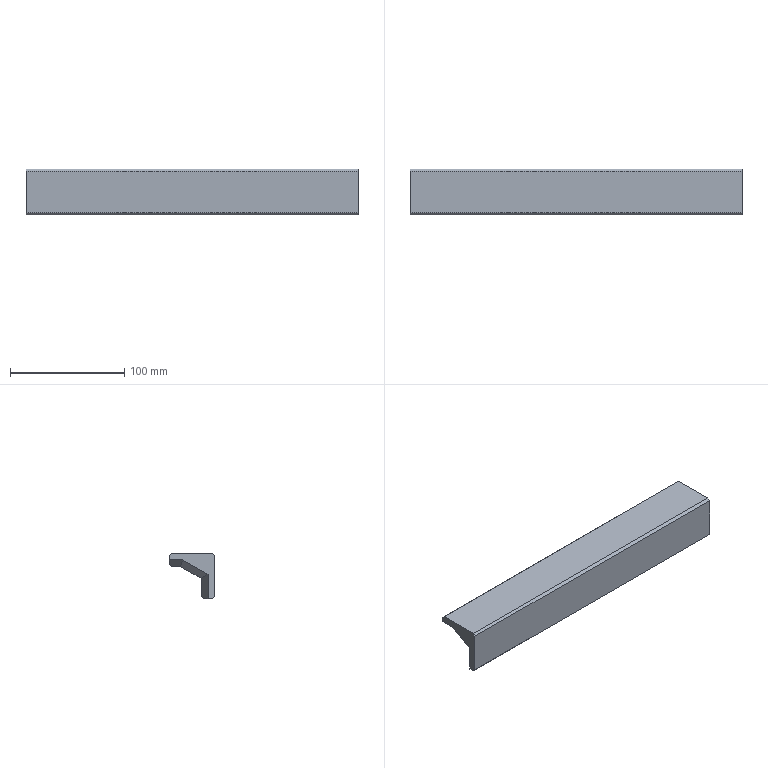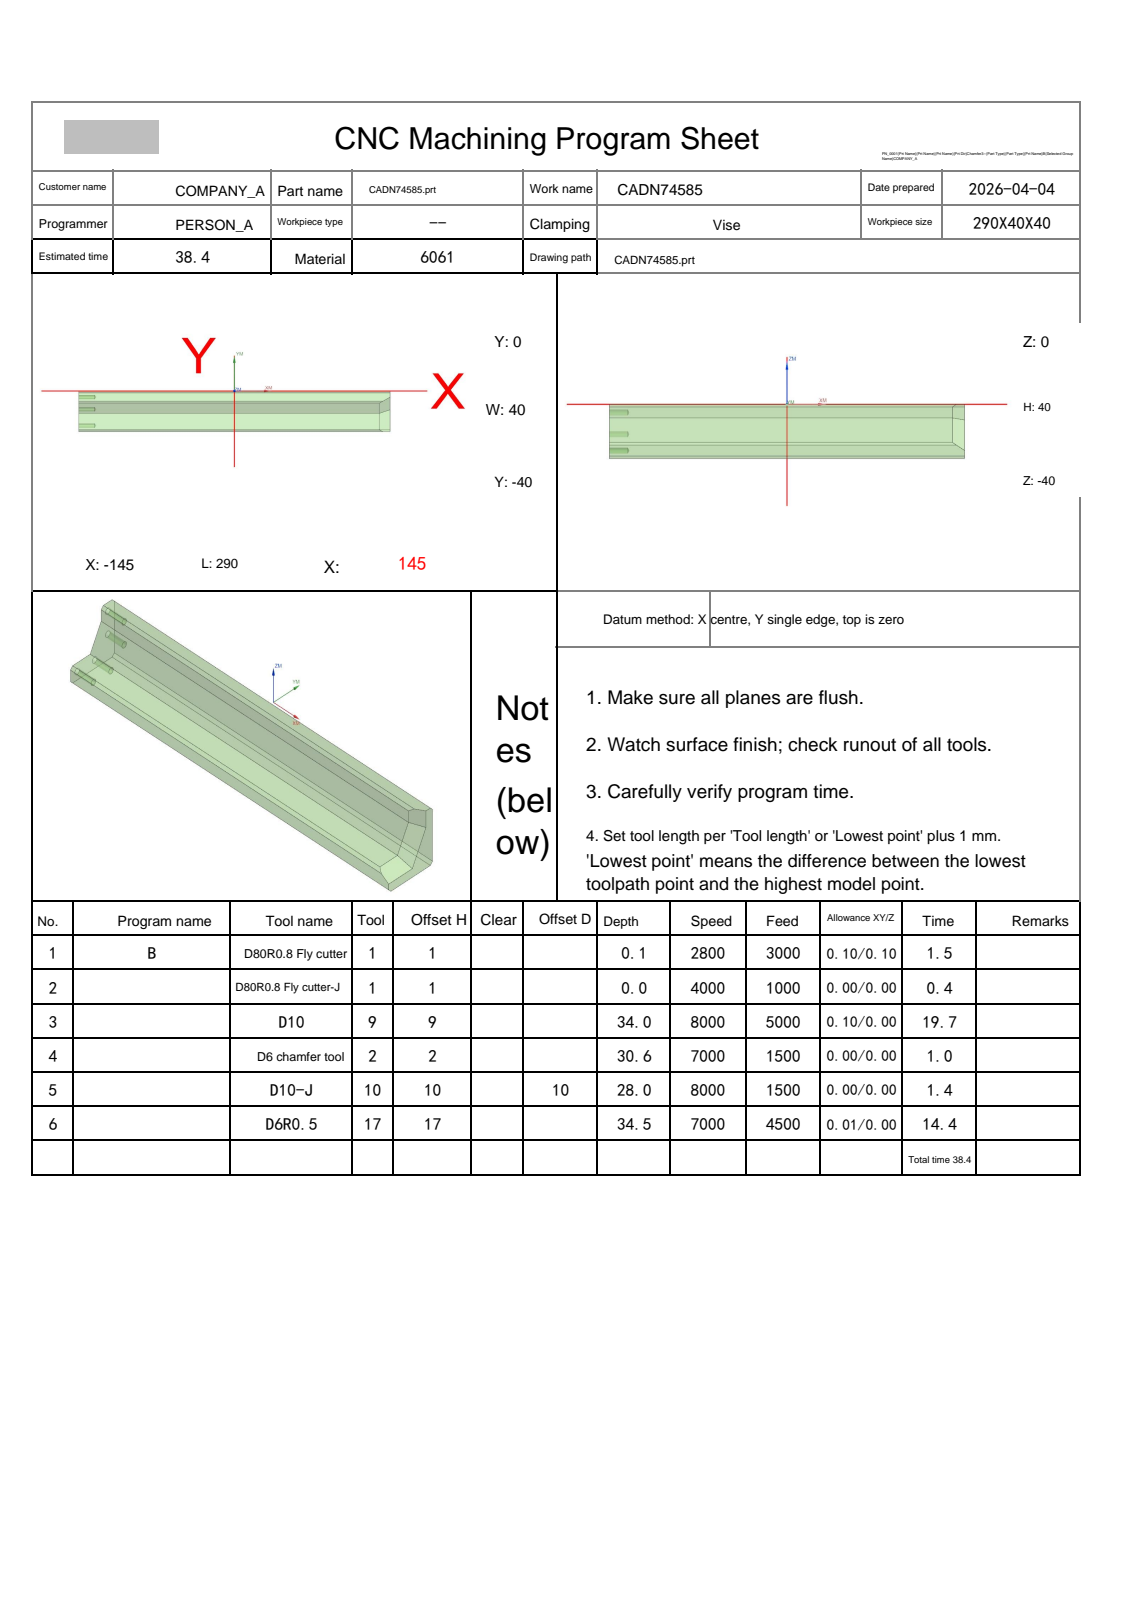NC program | NX | posted by the shop | part box 290 x 40 x 40 mm
Lines 110 to 1353 of 6846:
N3 T09 M06
(D10  D=10. R=0. H=09 ce=0.10 di=0.10)
G00 G90 G54 X8.423 Y-52.151 M03 S8000
G43 H09 Z14.5
M08
Z.702
G01 Z-.498 F5000.
Y-50.
G03 X1.423 Y-43. I-7. J0.0
G01 X-145.08
Y-42.864
Y-27.494
Y-27.051
Y-17.648
Y-17.039
Y-16.914
Y-15.639
X-138.08 Y-15.64
X137.385
G03 X140.127 Y-14.871 I-.14 J5.778
G01 X141. Y-14.348
X141.14 Y-14.264
X141.913 Y-13.8
X147.633 Y-10.368
G03 X147.945 Y-10.165 I-2.603 J4.338
G01 X147.961 Y-10.212
Y-11.804
Y-21.827
X147.994 Y-21.852
X148. Y-21.848
Y-40.08
X143.456
X143.382 Y-40.73
G02 X142.478 Y-43. I-5.022 J.686
G01 X-.563
G02 X-1.375 Y-42.582 I.001 J1.
G01 X-5.778 Y-36.418
G03 X-6.591 Y-36. I-.813 J-.582
G01 X-137.083
G02 X-138.08 Y-35.004 I.004 J1.
G01 Y-27.495
Y-27.052
Y-23.636
G02 X-137.084 Y-22.64 I1. J-.004
G01 X137.47
G03 X139.803 Y-22.383 I-.227 J12.778
G01 X140. Y-22.363
G02 X141. Y-23.359 I0.0 J-1.
G01 Y-32.868
G02 X140.435 Y-33.765 I-1. J.004
G03 X138.046 Y-35.638 I3.021 J-6.314
G02 X137.279 Y-36. I-.77 J.638
G01 X-.914
G02 X-1.619 Y-35.708 I.001 J1.
G01 X-5.534 Y-31.793
G03 X-6.241 Y-31.5 I-.707 J-.707
G01 X-132.584
G02 X-133.58 Y-30.504 I.004 J1.
G01 Y-28.135
G02 X-132.584 Y-27.14 I1. J-.004
G01 X135.504
G02 X136.5 Y-28.135 I-.004 J-1.
G01 Y-30.443
G02 X136.14 Y-31.207 I-1. J.004
G01 X136.065 Y-31.269
G02 X135.43 Y-31.5 I-.639 J.769
G01 X-3.577
X-4.077
G03 X-11.077 Y-38.5 I0.0 J-7.
G01 Y-52.151
Z.702
G00 Z3.
G01 X8.423 F6000.
G00 Z.204
G01 Z-.996 F5000.
Y-50.
G03 X1.423 Y-43. I-7. J0.0
G01 X-145.08
Y-42.864
Y-27.494
Y-27.051
Y-17.648
Y-16.914
Y-16.136
X-138.08 Y-16.138
X136.399
X136.45
G03 X139.297 Y-15.37 I0.0 J5.655
G01 X141. Y-14.348
X147.633 Y-10.368
G03 X147.945 Y-10.165 I-2.603 J4.338
G01 X147.961 Y-10.212
Y-11.804
Y-21.827
X147.994 Y-21.852
X148. Y-21.848
Y-40.08
X143.456
X143.382 Y-40.73
G02 X142.478 Y-43. I-5.022 J.686
G01 X-3.577
G02 X-4.548 Y-42.238 I0.0 J1.
G01 X-5.89 Y-36.761
G03 X-6.861 Y-36. I-.971 J-.239
G01 X-137.084
G02 X-138.08 Y-35.004 I.004 J1.
G01 Y-27.495
Y-27.052
Y-24.134
G02 X-137.084 Y-23.138 I1. J-.004
G01 X136.34
X136.45
G03 X139.744 Y-22.702 I0.0 J12.655
G02 X140. Y-22.669 I.256 J-.967
X141. Y-23.665 I0.0 J-1.
G01 Y-32.869
G02 X140.435 Y-33.765 I-1. J.004
G03 X138.046 Y-35.638 I3.021 J-6.315
G02 X137.28 Y-36. I-.77 J.638
G01 X-.914
G02 X-1.619 Y-35.708 I.001 J1.
G01 X-5.534 Y-31.793
G03 X-6.241 Y-31.5 I-.707 J-.707
G01 X-132.585
G02 X-133.58 Y-30.505 I.005 J1.
G01 Y-28.633
G02 X-132.585 Y-27.638 I1. J-.005
G01 X135.505
G02 X136.5 Y-28.633 I-.005 J-1.
G01 Y-30.443
G02 X136.14 Y-31.207 I-1. J.005
G01 X136.065 Y-31.269
G02 X135.431 Y-31.5 I-.639 J.769
G01 X-3.577
X-4.077
G03 X-11.077 Y-38.5 I0.0 J-7.
G01 Y-52.151
Z.204
G00 Z2.502
G01 X8.423 F6000.
G00 Z-.295
G01 Z-1.495 F5000.
Y-50.
G03 X1.423 Y-43. I-7. J0.0
G01 X-145.08
Y-42.864
Y-27.494
Y-27.051
Y-18.035
Y-17.648
Y-16.914
Y-16.634
X-138.08 Y-16.636
X135.724
G03 X138.466 Y-15.868 I-.016 J5.333
G01 X141. Y-14.348
X147.633 Y-10.368
G03 X147.945 Y-10.165 I-2.603 J4.338
G01 X147.948 Y-10.168
X147.961 Y-10.212
Y-11.804
Y-21.827
X147.994 Y-21.852
X148. Y-21.848
Y-40.08
X143.456
X143.382 Y-40.73
G02 X142.478 Y-43. I-5.022 J.686
G01 X-3.577
G02 X-4.548 Y-42.238 I0.0 J1.
G01 X-5.89 Y-36.761
G03 X-6.861 Y-36. I-.971 J-.239
G01 X-137.084
G02 X-138.08 Y-35.004 I.004 J1.
G01 Y-27.495
Y-27.052
Y-24.632
G02 X-137.084 Y-23.636 I1. J-.004
G01 X135.735
G03 X139.682 Y-22.978 I-.026 J12.333
G02 X140. Y-22.927 I.318 J-.948
X141. Y-23.922 I0.0 J-1.
G01 Y-32.869
G02 X140.436 Y-33.765 I-1. J.004
G03 X138.046 Y-35.638 I3.021 J-6.315
G02 X137.28 Y-36. I-.77 J.638
G01 X-.914
G02 X-1.619 Y-35.708 I.001 J1.
G01 X-5.534 Y-31.793
G03 X-6.241 Y-31.5 I-.707 J-.707
G01 X-132.585
G02 X-133.58 Y-30.505 I.005 J1.
G01 Y-29.131
G02 X-132.585 Y-28.136 I1. J-.005
G01 X135.505
G02 X136.5 Y-29.131 I-.005 J-1.
G01 Y-30.443
G02 X136.14 Y-31.207 I-1. J.005
G01 X136.065 Y-31.269
G02 X135.431 Y-31.5 I-.639 J.769
G01 X-3.577
X-4.077
G03 X-11.077 Y-38.5 I0.0 J-7.
G01 Y-52.151
Z-.295
G00 Z2.004
G01 X8.423 F6000.
G00 Z-.793
G01 Z-1.993 F5000.
Y-50.
G03 X1.423 Y-43. I-7. J0.0
G01 X-145.08
Y-42.864
Y-27.494
Y-27.051
Y-17.648
Y-17.449
Y-17.099
X-138.08 Y-17.1
X134.978
X134.983
G03 X137.636 Y-16.366 I0.0 J5.164
G01 X138.466 Y-15.868
X141. Y-14.348
X147.633 Y-10.368
G03 X147.945 Y-10.165 I-2.603 J4.338
G01 X147.961 Y-10.212
Y-11.804
Y-21.827
X147.994 Y-21.852
X148. Y-21.848
Y-40.08
X143.456
X143.382 Y-40.73
G02 X142.478 Y-43. I-5.022 J.686
G01 X-3.577
G02 X-4.548 Y-42.238 I0.0 J1.
G01 X-5.89 Y-36.761
G03 X-6.861 Y-36. I-.971 J-.239
G01 X-137.085
G02 X-138.08 Y-35.005 I.005 J1.
G01 Y-27.495
Y-27.052
Y-25.095
G02 X-137.085 Y-24.1 I1. J-.005
G01 X134.975
X134.983
G03 X139.623 Y-23.18 I0.0 J12.164
G02 X140. Y-23.106 I.377 J-.926
X141. Y-24.101 I0.0 J-1.
G01 Y-32.869
G02 X140.436 Y-33.765 I-1. J.005
G03 X138.046 Y-35.638 I3.02 J-6.315
G02 X137.28 Y-36. I-.77 J.638
G01 X-.914
G02 X-1.619 Y-35.708 I.001 J1.
G01 X-5.534 Y-31.793
G03 X-6.241 Y-31.5 I-.707 J-.707
G01 X-132.585
G02 X-133.58 Y-30.505 I.005 J1.
G01 Y-29.595
G02 X-132.585 Y-28.6 I1. J-.005
G01 X134.974
X134.983
G03 X135.476 Y-28.592 I0.0 J16.664
G01 X135.5
G02 X136.5 Y-29.587 I0.0 J-1.
G01 Y-30.444
G02 X136.14 Y-31.207 I-1. J.005
G01 X136.065 Y-31.27
G02 X135.431 Y-31.5 I-.639 J.77
G01 X-3.577
X-4.077
G03 X-11.077 Y-38.5 I0.0 J-7.
G01 Y-52.151
Z-.793
G00 Z1.505
G01 X8.423 F6000.
G00 Z-1.291
G01 Z-2.491 F5000.
Y-50.
G03 X1.423 Y-43. I-7. J0.0
G01 X-145.08
Y-42.864
Y-27.494
Y-27.051
Y-17.648
Y-17.099
X-138.08 Y-17.1
X135.
G03 X137.624 Y-16.373 I0.0 J5.1
G01 X141. Y-14.348
X147.633 Y-10.368
G03 X147.945 Y-10.165 I-2.603 J4.338
G01 X147.961 Y-10.212
Y-11.804
Y-21.827
X147.994 Y-21.852
X148. Y-21.848
Y-40.08
X143.456
X143.382 Y-40.73
G02 X142.478 Y-43. I-5.022 J.686
G01 X-3.577
G02 X-4.548 Y-42.238 I0.0 J1.
G01 X-5.89 Y-36.761
G03 X-6.861 Y-36. I-.971 J-.239
G01 X-137.085
G02 X-138.08 Y-35.005 I.005 J1.
G01 Y-27.495
Y-25.095
G02 X-137.085 Y-24.1 I1. J-.005
G01 X135.
G03 X139.623 Y-23.182 I0.0 J12.1
G02 X140. Y-23.108 I.377 J-.926
X141. Y-24.103 I0.0 J-1.
G01 Y-32.87
G02 X140.436 Y-33.765 I-1. J.005
G03 X138.045 Y-35.638 I3.02 J-6.315
G02 X137.281 Y-36. I-.77 J.638
G01 X-.914
G02 X-1.619 Y-35.708 I.001 J1.
G01 X-5.534 Y-31.793
G03 X-6.241 Y-31.5 I-.707 J-.707
G01 X-132.585
G02 X-133.58 Y-30.505 I.005 J1.
G01 Y-29.595
G02 X-132.585 Y-28.6 I1. J-.005
G01 X135.
G03 X135.477 Y-28.593 I0.0 J16.6
G01 X135.5
G02 X136.5 Y-29.587 I0.0 J-1.
G01 Y-30.444
G02 X136.141 Y-31.207 I-1. J.005
G01 X136.065 Y-31.27
G02 X135.432 Y-31.5 I-.638 J.77
G01 X-3.577
X-4.077
G03 X-11.077 Y-38.5 I0.0 J-7.
G01 Y-52.151
Z-1.291
G00 Z1.007
G01 X8.423 F6000.
G00 Z-1.789
G01 Z-2.989 F5000.
Y-50.
G03 X1.423 Y-43. I-7. J0.0
G01 X-145.08
Y-42.864
Y-27.494
Y-27.051
Y-24.1
Y-17.647
Y-17.099
X-138.08 Y-17.1
X135.
X135.208 Y-17.096
G03 X137.624 Y-16.373 I-.208 J5.096
G01 X141. Y-14.348
X147.633 Y-10.368
G03 X147.945 Y-10.165 I-2.603 J4.338
G01 X147.961 Y-10.212
Y-11.804
Y-21.827
X147.994 Y-21.852
X148. Y-21.848
Y-40.08
X143.456
X143.382 Y-40.73
G02 X142.478 Y-43. I-5.022 J.686
G01 X-3.577
G02 X-4.548 Y-42.238 I0.0 J1.
G01 X-5.89 Y-36.761
G03 X-6.861 Y-36. I-.971 J-.239
G01 X-137.085
G02 X-138.08 Y-35.005 I.005 J1.
G01 Y-27.495
Y-27.052
Y-25.095
G02 X-137.085 Y-24.1 I1. J-.005
G01 X135.493 Y-24.09
G03 X139.623 Y-23.182 I-.493 J12.09
G02 X140. Y-23.108 I.377 J-.926
X141. Y-24.103 I0.0 J-1.
G01 Y-32.87
G02 X140.436 Y-33.764 I-1. J.005
G03 X138.045 Y-35.639 I3.02 J-6.315
G02 X137.281 Y-36. I-.769 J.639
G01 X-.914
G02 X-1.619 Y-35.708 I.001 J1.
G01 X-5.534 Y-31.793
G03 X-6.241 Y-31.5 I-.707 J-.707
G01 X-132.586
G02 X-133.58 Y-30.506 I.006 J1.
G01 Y-29.594
G02 X-132.586 Y-28.6 I1. J-.006
G01 X135.506 Y-28.59
G02 X136.5 Y-29.584 I-.006 J-1.
G01 Y-30.444
G02 X136.141 Y-31.206 I-1. J.006
G01 X136.064 Y-31.27
G02 X135.432 Y-31.5 I-.638 J.77
G01 X-3.577
X-4.077
G03 X-11.077 Y-38.5 I0.0 J-7.
G01 Y-52.151
Z-1.789
G00 Z.509
G01 X8.423 F6000.
G00 Z-2.288
G01 Z-3.488 F5000.
Y-50.
G03 X1.423 Y-43. I-7. J0.0
G01 X-145.08
Y-42.864
Y-27.494
Y-27.051
Y-17.648
Y-17.099
X-138.08 Y-17.1
X135.
G03 X137.624 Y-16.373 I0.0 J5.1
G01 X141. Y-14.348
X147.633 Y-10.368
G03 X147.945 Y-10.165 I-2.603 J4.338
G01 X147.948 Y-10.168
X147.961 Y-10.212
Y-11.804
Y-21.827
X147.994 Y-21.852
X148. Y-21.848
Y-40.08
X143.456
X143.382 Y-40.73
G02 X142.478 Y-43. I-5.022 J.686
G01 X-3.577
G02 X-4.548 Y-42.238 I0.0 J1.
G01 X-5.89 Y-36.761
G03 X-6.861 Y-36. I-.971 J-.239
G01 X-137.085
G02 X-138.08 Y-35.005 I.005 J1.
G01 Y-27.495
Y-27.052
Y-25.095
G02 X-137.085 Y-24.1 I1. J-.005
G01 X135.
G03 X139.623 Y-23.182 I0.0 J12.1
G02 X140. Y-23.108 I.377 J-.926
X141. Y-24.103 I0.0 J-1.
G01 Y-32.87
G02 X140.437 Y-33.764 I-1. J.005
G03 X138.045 Y-35.639 I3.02 J-6.315
G02 X137.281 Y-36. I-.769 J.639
G01 X-.914
G02 X-1.619 Y-35.708 I.001 J1.
G01 X-5.534 Y-31.793
G03 X-6.241 Y-31.5 I-.707 J-.707
G01 X-132.586
G02 X-133.58 Y-30.506 I.006 J1.
G01 Y-29.594
G02 X-132.586 Y-28.6 I1. J-.006
G01 X135.
G03 X135.477 Y-28.593 I0.0 J16.6
G01 X135.5
G02 X136.5 Y-29.587 I0.0 J-1.
G01 Y-30.445
G02 X136.141 Y-31.206 I-1. J.006
G01 X136.064 Y-31.27
G02 X135.432 Y-31.5 I-.638 J.77
G01 X-3.577
X-4.077
G03 X-11.077 Y-38.5 I0.0 J-7.
G01 Y-52.151
Z-2.288
G00 Z.011
G01 X8.423 F6000.
G00 Z-2.786
G01 Z-3.986 F5000.
Y-50.
G03 X1.423 Y-43. I-7. J0.0
G01 X-145.08
Y-42.864
Y-27.494
Y-27.051
Y-17.648
Y-17.099
X-138.08 Y-17.1
X135.
G03 X137.624 Y-16.373 I0.0 J5.1
G01 X141. Y-14.348
X147.633 Y-10.368
G03 X147.945 Y-10.165 I-2.603 J4.338
G01 X147.948 Y-10.168
X147.961 Y-10.212
Y-11.804
Y-21.827
X147.994 Y-21.852
X148. Y-21.848
Y-40.08
X143.456
X143.382 Y-40.73
G02 X142.478 Y-43. I-5.022 J.686
G01 X-3.577
G02 X-4.548 Y-42.238 I0.0 J1.
G01 X-5.89 Y-36.761
G03 X-6.861 Y-36. I-.971 J-.239
G01 X-137.086
G02 X-138.08 Y-35.006 I.006 J1.
G01 Y-27.495
Y-27.052
Y-25.094
G02 X-137.086 Y-24.1 I1. J-.006
G01 X135.
G03 X139.623 Y-23.182 I0.0 J12.1
G02 X140. Y-23.108 I.377 J-.926
X141. Y-24.103 I0.0 J-1.
G01 Y-32.87
G02 X140.437 Y-33.764 I-1. J.006
G03 X138.045 Y-35.639 I3.019 J-6.315
G02 X137.281 Y-36. I-.769 J.639
G01 X-.914
G02 X-1.619 Y-35.708 I.001 J1.
G01 X-5.534 Y-31.793
G03 X-6.241 Y-31.5 I-.707 J-.707
G01 X-132.586
G02 X-133.58 Y-30.506 I.006 J1.
G01 Y-29.594
G02 X-132.586 Y-28.6 I1. J-.006
G01 X135.
G03 X135.478 Y-28.593 I0.0 J16.6
G01 X135.5
G02 X136.5 Y-29.587 I0.0 J-1.
G01 Y-30.445
G02 X136.141 Y-31.206 I-1. J.006
G01 X136.064 Y-31.27
G02 X135.432 Y-31.5 I-.638 J.77
G01 X-3.577
X-4.077
G03 X-11.077 Y-38.5 I0.0 J-7.
G01 Y-52.151
Z-2.786
G00 Z-.488
G01 X8.423 F6000.
G00 Z-3.284
G01 Z-4.484 F5000.
Y-50.
G03 X1.423 Y-43. I-7. J0.0
G01 X-145.08
Y-42.864
Y-27.494
Y-27.051
Y-17.648
Y-17.099
X-138.08 Y-17.1
X135.
G03 X137.624 Y-16.373 I0.0 J5.1
G01 X141. Y-14.348
X147.633 Y-10.368
G03 X147.945 Y-10.165 I-2.603 J4.338
G01 X147.948 Y-10.168
X147.961 Y-10.212
Y-11.804
Y-21.827
X147.994 Y-21.852
X148. Y-21.848
Y-40.08
X143.456
X143.382 Y-40.73
G02 X142.478 Y-43. I-5.022 J.686
G01 X-3.577
G02 X-4.548 Y-42.238 I0.0 J1.
G01 X-5.89 Y-36.761
G03 X-6.861 Y-36. I-.971 J-.239
G01 X-137.086
G02 X-138.08 Y-35.006 I.006 J1.
G01 Y-27.495
Y-27.052
Y-25.094
G02 X-137.086 Y-24.1 I1. J-.006
G01 X135.
G03 X139.624 Y-23.182 I0.0 J12.1
G02 X140. Y-23.108 I.376 J-.926
X141. Y-24.102 I0.0 J-1.
G01 Y-32.871
G02 X140.437 Y-33.764 I-1. J.006
G03 X138.045 Y-35.639 I3.019 J-6.315
G02 X137.282 Y-36. I-.769 J.639
G01 X-.914
G02 X-1.619 Y-35.708 I.001 J1.
G01 X-5.534 Y-31.793
G03 X-6.241 Y-31.5 I-.707 J-.707
G01 X-132.586
G02 X-133.58 Y-30.506 I.006 J1.
G01 Y-29.594
G02 X-132.586 Y-28.6 I1. J-.006
G01 X135.
G03 X135.478 Y-28.593 I0.0 J16.6
G01 X135.5
G02 X136.5 Y-29.586 I0.0 J-1.
G01 Y-30.445
G02 X136.141 Y-31.206 I-1. J.006
G01 X136.064 Y-31.27
G02 X135.433 Y-31.5 I-.638 J.77
G01 X-3.577
X-4.077
G03 X-11.077 Y-38.5 I0.0 J-7.
G01 Y-52.151
Z-3.284
G00 Z-.986
G01 X8.423 F6000.
G00 Z-3.782
G01 Z-4.982 F5000.
Y-50.
G03 X1.423 Y-43. I-7. J0.0
G01 X-145.08
Y-42.864
Y-27.494
Y-27.051
Y-18.303
Y-17.648
Y-17.099
X-138.08 Y-17.1
X135.
G03 X137.624 Y-16.373 I0.0 J5.1
G01 X141. Y-14.348
X147.633 Y-10.368
G03 X147.945 Y-10.165 I-2.603 J4.338
G01 X147.961 Y-10.212
Y-11.804
Y-21.827
X147.994 Y-21.852
X148. Y-21.848
Y-40.08
X143.456
X143.382 Y-40.73
G02 X142.478 Y-43. I-5.022 J.686
G01 X-3.577
G02 X-4.548 Y-42.238 I0.0 J1.
G01 X-5.89 Y-36.761
G03 X-6.861 Y-36. I-.971 J-.239
G01 X-137.086
G02 X-138.08 Y-35.006 I.006 J1.
G01 Y-27.495
Y-27.052
Y-25.094
G02 X-137.086 Y-24.1 I1. J-.006
G01 X135.
G03 X139.624 Y-23.182 I0.0 J12.1
G02 X140. Y-23.108 I.376 J-.927
X141. Y-24.102 I0.0 J-1.
G01 Y-32.871
G02 X140.437 Y-33.764 I-1. J.006
G03 X138.045 Y-35.639 I3.019 J-6.316
G02 X137.282 Y-36. I-.769 J.639
G01 X-.914
G02 X-1.619 Y-35.708 I.001 J1.
G01 X-5.534 Y-31.793
G03 X-6.241 Y-31.5 I-.707 J-.707
G01 X-132.587
G02 X-133.58 Y-30.507 I.007 J1.
G01 Y-29.593
G02 X-132.587 Y-28.6 I1. J-.007
G01 X135.
G03 X135.478 Y-28.593 I0.0 J16.6
G01 X135.5
G02 X136.5 Y-29.586 I0.0 J-1.
G01 Y-30.445
G02 X136.141 Y-31.206 I-1. J.007
G01 X136.064 Y-31.27
G02 X135.433 Y-31.5 I-.638 J.77
G01 X-3.577
X-4.077
G03 X-11.077 Y-38.5 I0.0 J-7.
G01 Y-52.151
Z-3.782
G00 Z-1.484
G01 X8.423 F6000.
G00 Z-4.28
G01 Z-5.48 F5000.
Y-50.
G03 X1.423 Y-43. I-7. J0.0
G01 X-145.08
Y-42.864
Y-27.494
Y-27.051
Y-17.648
Y-17.099
X-138.08 Y-17.1
X135.
G03 X137.624 Y-16.373 I0.0 J5.1
G01 X141. Y-14.348
X147.633 Y-10.368
G03 X147.945 Y-10.165 I-2.603 J4.338
G01 X147.948 Y-10.168
X147.961 Y-10.212
Y-11.804
Y-21.827
X147.994 Y-21.852
X148. Y-21.848
Y-40.08
X143.456
X143.382 Y-40.73
G02 X142.478 Y-43. I-5.022 J.686
G01 X-3.577
G02 X-4.548 Y-42.238 I0.0 J1.
G01 X-5.89 Y-36.761
G03 X-6.861 Y-36. I-.971 J-.239
G01 X-137.086
G02 X-138.08 Y-35.006 I.006 J1.
G01 Y-27.495
Y-27.052
Y-25.094
G02 X-137.086 Y-24.1 I1. J-.006
G01 X135.
G03 X139.624 Y-23.182 I0.0 J12.1
G02 X140. Y-23.108 I.376 J-.927
X141. Y-24.102 I0.0 J-1.
G01 Y-32.871
G02 X140.437 Y-33.764 I-1. J.006
G03 X138.045 Y-35.64 I3.019 J-6.316
G02 X137.282 Y-36. I-.769 J.64
G01 X-.914
G02 X-1.619 Y-35.708 I.001 J1.
G01 X-5.534 Y-31.793
G03 X-6.241 Y-31.5 I-.707 J-.707
G01 X-132.587
G02 X-133.58 Y-30.507 I.007 J1.
G01 Y-29.593
G02 X-132.587 Y-28.6 I1. J-.007
G01 X135.
G03 X135.478 Y-28.593 I0.0 J16.6
G01 X135.5
G02 X136.5 Y-29.586 I0.0 J-1.
G01 Y-30.445
G02 X136.142 Y-31.206 I-1. J.007
G01 X136.064 Y-31.271
G02 X135.433 Y-31.5 I-.637 J.771
G01 X-3.577
X-4.077
G03 X-11.077 Y-38.5 I0.0 J-7.
G01 Y-52.151
Z-4.28
G00 Z-1.982
G01 X8.423 F6000.
G00 Z-4.779
G01 Z-5.979 F5000.
Y-50.
G03 X1.423 Y-43. I-7. J0.0
G01 X-145.08
Y-42.864
Y-27.494
Y-27.051
Y-17.648
Y-17.099
X-138.08 Y-17.1
X135.
G03 X137.624 Y-16.373 I0.0 J5.1
G01 X141. Y-14.348
X147.633 Y-10.368
G03 X147.945 Y-10.165 I-2.603 J4.338
G01 X147.961 Y-10.212
Y-11.804
Y-21.827
X147.994 Y-21.852
X148. Y-21.848
Y-40.08
X143.456
X143.382 Y-40.73
G02 X142.478 Y-43. I-5.022 J.686
G01 X-3.577
G02 X-4.548 Y-42.238 I0.0 J1.
G01 X-5.89 Y-36.761
G03 X-6.861 Y-36. I-.971 J-.239
G01 X-137.087
G02 X-138.08 Y-35.007 I.007 J1.
G01 Y-27.495
Y-25.093
G02 X-137.087 Y-24.1 I1. J-.007
G01 X135.
G03 X139.624 Y-23.182 I0.0 J12.1
G02 X140. Y-23.108 I.376 J-.927
X141. Y-24.102 I0.0 J-1.
G01 Y-32.871
G02 X140.438 Y-33.764 I-1. J.007
G03 X138.044 Y-35.64 I3.019 J-6.316
G02 X137.282 Y-36. I-.769 J.64
G01 X-.914
G02 X-1.619 Y-35.708 I.001 J1.
G01 X-5.534 Y-31.793
G03 X-6.241 Y-31.5 I-.707 J-.707
G01 X-132.587
G02 X-133.58 Y-30.507 I.007 J1.
G01 Y-29.593
G02 X-132.587 Y-28.6 I1. J-.007
G01 X135.
G03 X135.478 Y-28.593 I0.0 J16.6
G01 X135.5
G02 X136.5 Y-29.586 I0.0 J-1.
G01 Y-30.446
G02 X136.142 Y-31.206 I-1. J.007
G01 X136.063 Y-31.271
G02 X135.433 Y-31.5 I-.637 J.771
G01 X-3.577
X-4.077
G03 X-11.077 Y-38.5 I0.0 J-7.
G01 Y-52.151
Z-4.779
G00 Z-2.48
G01 X8.423 F6000.
G00 Z-5.277
G01 Z-6.477 F5000.
Y-50.
G03 X1.423 Y-43. I-7. J0.0
G01 X-145.08
Y-42.864
Y-27.494
Y-27.051
Y-17.648
Y-17.099
X-138.08 Y-17.1
X135.
G03 X137.624 Y-16.373 I0.0 J5.1
G01 X141. Y-14.348
X147.633 Y-10.368
G03 X147.945 Y-10.165 I-2.603 J4.338
G01 X147.961 Y-10.212
Y-11.804
Y-21.827
X147.994 Y-21.852
X148. Y-21.848
Y-40.08
X143.456
X143.382 Y-40.73
G02 X142.478 Y-43. I-5.022 J.686
G01 X-3.577
G02 X-4.548 Y-42.238 I0.0 J1.
G01 X-5.89 Y-36.761
G03 X-6.861 Y-36. I-.971 J-.239
G01 X-137.087
G02 X-138.08 Y-35.007 I.007 J1.
G01 Y-27.495
Y-25.093
G02 X-137.087 Y-24.1 I1. J-.007
G01 X135.
G03 X139.624 Y-23.181 I0.0 J12.1
G02 X140. Y-23.108 I.376 J-.927
X141. Y-24.101 I0.0 J-1.
G01 Y-32.872
G02 X140.438 Y-33.764 I-1. J.007
G03 X138.044 Y-35.64 I3.018 J-6.316
G02 X137.283 Y-36. I-.768 J.64
G01 X-.914
G02 X-1.619 Y-35.708 I.001 J1.
G01 X-5.534 Y-31.793
G03 X-6.241 Y-31.5 I-.707 J-.707
G01 X-132.587
G02 X-133.58 Y-30.507 I.007 J1.
G01 Y-29.593
G02 X-132.587 Y-28.6 I1. J-.007
G01 X135.
G03 X135.479 Y-28.593 I0.0 J16.6
G01 X135.5
G02 X136.5 Y-29.585 I0.0 J-1.
G01 Y-30.446
G02 X136.142 Y-31.205 I-1. J.007
G01 X136.063 Y-31.271
G02 X135.434 Y-31.5 I-.637 J.771
G01 X-3.577
X-4.077
G03 X-11.077 Y-38.5 I0.0 J-7.
G01 Y-52.151
Z-5.277
G00 Z-2.979
G01 X8.423 F6000.
G00 Z-5.775
G01 Z-6.975 F5000.
Y-50.
G03 X1.423 Y-43. I-7. J0.0
G01 X-145.08
Y-42.864
Y-27.494
Y-27.051
Y-17.648
Y-17.1
X-138.08
X135.
G03 X137.624 Y-16.373 I0.0 J5.1
G01 X141. Y-14.348
X147.633 Y-10.368
G03 X147.945 Y-10.165 I-2.603 J4.338
G01 X147.948 Y-10.168
X147.961 Y-10.212
Y-21.827
X147.994 Y-21.852
X148. Y-21.848
Y-40.08
X143.456
X143.382 Y-40.73
G02 X142.478 Y-43. I-5.022 J.686
G01 X-3.577
G02 X-4.548 Y-42.238 I0.0 J1.
G01 X-5.89 Y-36.761
G03 X-6.861 Y-36. I-.971 J-.239
G01 X-137.087
G02 X-138.08 Y-35.007 I.007 J1.
G01 Y-27.495
Y-27.052
Y-25.093
G02 X-137.087 Y-24.1 I1. J-.007
G01 X135.
G03 X139.625 Y-23.181 I0.0 J12.1
G02 X140. Y-23.108 I.375 J-.927
X141. Y-24.101 I0.0 J-1.
G01 Y-32.872
G02 X140.438 Y-33.764 I-1. J.007
G03 X138.044 Y-35.64 I3.018 J-6.316
G02 X137.283 Y-36. I-.768 J.64
G01 X-.914
G02 X-1.619 Y-35.708 I.001 J1.
G01 X-5.534 Y-31.793
G03 X-6.241 Y-31.5 I-.707 J-.707
G01 X-132.587
G02 X-133.58 Y-30.507 I.007 J1.
G01 Y-29.593
G02 X-132.587 Y-28.6 I1. J-.007
G01 X135.
G03 X135.479 Y-28.593 I0.0 J16.6
G01 X135.5
G02 X136.5 Y-29.585 I0.0 J-1.
G01 Y-30.446
G02 X136.142 Y-31.205 I-1. J.007
G01 X136.063 Y-31.271
G02 X135.434 Y-31.5 I-.637 J.771
G01 X-3.577
X-4.077
G03 X-11.077 Y-38.5 I0.0 J-7.
G01 Y-52.151
Z-5.775
G00 Z-3.477
G01 X8.423 F6000.
G00 Z-6.273
G01 Z-7.473 F5000.
Y-50.
G03 X1.423 Y-43. I-7. J0.0
G01 X-145.08
Y-42.864
Y-27.494
Y-27.051
Y-18.303
Y-17.648
Y-17.099
X-138.08 Y-17.1
X135.
G03 X137.624 Y-16.373 I0.0 J5.1
G01 X141.47 Y-14.066
X147.633 Y-10.368
G03 X147.945 Y-10.165 I-2.603 J4.338
G01 X147.961 Y-10.212
Y-21.827
X147.994 Y-21.852
X148. Y-21.848
Y-40.08
X143.456
X143.382 Y-40.73
G02 X142.478 Y-43. I-5.022 J.686
G01 X-3.577
G02 X-4.548 Y-42.238 I0.0 J1.
G01 X-5.89 Y-36.761
G03 X-6.861 Y-36. I-.971 J-.239
G01 X-137.087
G02 X-138.08 Y-35.007 I.007 J1.
G01 Y-27.495
Y-27.052
Y-25.093
G02 X-137.087 Y-24.1 I1. J-.007
G01 X135.
G03 X139.625 Y-23.181 I0.0 J12.1
G02 X140. Y-23.108 I.375 J-.927
X141. Y-24.101 I0.0 J-1.
G01 Y-32.872
G02 X140.438 Y-33.764 I-1. J.007
G03 X138.044 Y-35.64 I3.018 J-6.316
G02 X137.283 Y-36. I-.768 J.64
G01 X-.914
G02 X-1.619 Y-35.708 I.001 J1.
G01 X-5.534 Y-31.793
G03 X-6.241 Y-31.5 I-.707 J-.707
G01 X-132.588
G02 X-133.58 Y-30.508 I.008 J1.
G01 Y-29.592
G02 X-132.588 Y-28.6 I1. J-.008
G01 X135.
G03 X135.479 Y-28.593 I0.0 J16.6
G01 X135.5
G02 X136.5 Y-29.585 I0.0 J-1.
G01 Y-30.446
G02 X136.142 Y-31.205 I-1. J.008
G01 X136.063 Y-31.271
G02 X135.434 Y-31.5 I-.637 J.771
G01 X-3.577
X-4.077
G03 X-11.077 Y-38.5 I0.0 J-7.
G01 Y-52.151
Z-6.273
G00 Z-3.975
G01 X8.423 F6000.
G00 Z-6.771
G01 Z-7.971 F5000.
Y-50.
G03 X1.423 Y-43. I-7. J0.0
G01 X-145.08
Y-42.864
Y-27.494
Y-27.051
Y-17.648
Y-17.099
X-138.08 Y-17.1
X135.
G03 X137.624 Y-16.373 I0.0 J5.1
G01 X141. Y-14.348
X147.633 Y-10.368
G03 X147.945 Y-10.165 I-2.603 J4.338
G01 X147.948 Y-10.168
X147.961 Y-10.212
Y-11.804
Y-21.827
X147.994 Y-21.852
X148. Y-21.848
Y-40.08
X143.456
X143.382 Y-40.73
G02 X142.478 Y-43. I-5.022 J.686
G01 X-3.577
G02 X-4.548 Y-42.238 I0.0 J1.
G01 X-5.89 Y-36.761
G03 X-6.861 Y-36. I-.971 J-.239
G01 X-137.087
G02 X-138.08 Y-35.007 I.007 J1.
G01 Y-27.495
Y-25.093
G02 X-137.087 Y-24.1 I1. J-.007
G01 X135.
G03 X139.625 Y-23.181 I0.0 J12.1
G02 X140. Y-23.108 I.375 J-.927
X141. Y-24.101 I0.0 J-1.
G01 Y-32.872
G02 X140.438 Y-33.764 I-1. J.007
G03 X138.044 Y-35.64 I3.018 J-6.316
G02 X137.283 Y-36. I-.768 J.64
G01 X-.914
G02 X-1.619 Y-35.708 I.001 J1.
G01 X-5.534 Y-31.793
G03 X-6.241 Y-31.5 I-.707 J-.707
G01 X-132.588
G02 X-133.58 Y-30.508 I.008 J1.
G01 Y-29.592
G02 X-132.588 Y-28.6 I1. J-.008
G01 X135.
G03 X135.479 Y-28.593 I0.0 J16.6
G01 X135.5
G02 X136.5 Y-29.585 I0.0 J-1.
G01 Y-30.447
G02 X136.142 Y-31.205 I-1. J.008
G01 X136.063 Y-31.271
G02 X135.434 Y-31.5 I-.637 J.771
G01 X-3.577
X-4.077
G03 X-11.077 Y-38.5 I0.0 J-7.
G01 Y-52.151
Z-6.771
G00 Z-4.473
G01 X8.423 F6000.
G00 Z-7.27
G01 Z-8.47 F5000.
Y-50.
G03 X1.423 Y-43. I-7. J0.0
G01 X-145.08
Y-42.864
Y-27.494
Y-27.051
Y-17.648
Y-17.099
X-138.08 Y-17.1
X135.
G03 X137.624 Y-16.373 I0.0 J5.1
G01 X141. Y-14.348
X147.633 Y-10.368
G03 X147.945 Y-10.165 I-2.603 J4.338
G01 X147.961 Y-10.212
Y-21.827
X147.994 Y-21.852
X148. Y-21.848
Y-40.08
X143.456
X143.382 Y-40.73
G02 X142.478 Y-43. I-5.022 J.686
G01 X-3.577
G02 X-4.548 Y-42.238 I0.0 J1.
G01 X-5.89 Y-36.761
G03 X-6.861 Y-36. I-.971 J-.239
G01 X-137.088
G02 X-138.08 Y-35.008 I.008 J1.
G01 Y-27.495
Y-25.092
G02 X-137.088 Y-24.1 I1. J-.008
G01 X135.
G03 X139.625 Y-23.181 I0.0 J12.1
G02 X140. Y-23.108 I.375 J-.927
X141. Y-24.101 I0.0 J-1.
G01 Y-32.872
G02 X140.438 Y-33.763 I-1. J.008
G03 X138.044 Y-35.64 I3.018 J-6.316
G02 X137.283 Y-36. I-.768 J.64
G01 X-.914
G02 X-1.619 Y-35.708 I.001 J1.
G01 X-5.534 Y-31.793
G03 X-6.241 Y-31.5 I-.707 J-.707
G01 X-132.588
G02 X-133.58 Y-30.508 I.008 J1.
G01 Y-29.592
G02 X-132.588 Y-28.6 I1. J-.008
G01 X135.
G03 X135.479 Y-28.593 I0.0 J16.6
G01 X135.5
G02 X136.5 Y-29.585 I0.0 J-1.
G01 Y-30.447
G02 X136.142 Y-31.205 I-1. J.008
G01 X136.063 Y-31.271
G02 X135.434 Y-31.5 I-.637 J.771
G01 X-3.577
X-4.077
G03 X-11.077 Y-38.5 I0.0 J-7.
G01 Y-52.151
Z-7.27
G00 Z-4.971
G01 X8.423 F6000.
G00 Z-7.768
G01 Z-8.968 F5000.
Y-50.
G03 X1.423 Y-43. I-7. J0.0
G01 X-145.08
Y-42.864
Y-27.494
Y-27.051
Y-17.648
Y-17.099
X-138.08 Y-17.1
X135.
G03 X137.624 Y-16.373 I0.0 J5.1
G01 X141. Y-14.348
X147.633 Y-10.368
G03 X147.945 Y-10.165 I-2.603 J4.338
G01 X147.948 Y-10.168
X147.961 Y-10.212
Y-11.804
Y-21.827
X147.994 Y-21.852
X148. Y-21.848
Y-40.08
X143.456
X143.382 Y-40.73
G02 X142.478 Y-43. I-5.022 J.686
G01 X-3.577
G02 X-4.548 Y-42.238 I0.0 J1.
G01 X-5.89 Y-36.761
G03 X-6.861 Y-36. I-.971 J-.239
G01 X-137.088
G02 X-138.08 Y-35.008 I.008 J1.
G01 Y-27.495
Y-25.092
G02 X-137.088 Y-24.1 I1. J-.008
G01 X135.
G03 X139.625 Y-23.181 I0.0 J12.1
G02 X140. Y-23.108 I.375 J-.927
X141. Y-24.1 I0.0 J-1.
G01 Y-32.873
G02 X140.439 Y-33.763 I-1. J.008
G03 X138.044 Y-35.641 I3.018 J-6.316
G02 X137.284 Y-36. I-.768 J.641
G01 X-.914
G02 X-1.619 Y-35.708 I.001 J1.
G01 X-5.534 Y-31.793
G03 X-6.241 Y-31.5 I-.707 J-.707
G01 X-132.588
G02 X-133.58 Y-30.508 I.008 J1.
G01 Y-29.592
G02 X-132.588 Y-28.6 I1. J-.008
G01 X135.
G03 X135.48 Y-28.593 I0.0 J16.6
G01 X135.5
G02 X136.5 Y-29.585 I0.0 J-1.
G01 Y-30.447
G02 X136.143 Y-31.205 I-1. J.008
G01 X136.063 Y-31.271
G02 X135.434 Y-31.5 I-.636 J.771
G01 X-3.577
X-4.077
G03 X-11.077 Y-38.5 I0.0 J-7.
G01 Y-52.151
Z-7.768
G00 Z-5.47
G01 X8.423 F6000.
G00 Z-8.266
G01 Z-9.466 F5000.
Y-50.
G03 X1.423 Y-43. I-7. J0.0
G01 X-145.08
Y-42.864
Y-27.494
Y-27.051
Y-17.648
Y-17.099
X-138.08 Y-17.1
X135.
G03 X137.624 Y-16.373 I0.0 J5.1
G01 X141. Y-14.348
X147.633 Y-10.368
G03 X147.945 Y-10.165 I-2.603 J4.338
G01 X147.948 Y-10.168
X147.961 Y-10.212
Y-11.804
Y-21.827
X147.994 Y-21.852
X148. Y-21.848
Y-40.08
X143.456
X143.382 Y-40.73
G02 X142.478 Y-43. I-5.022 J.686
G01 X-3.577
G02 X-4.548 Y-42.238 I0.0 J1.
G01 X-5.89 Y-36.761
G03 X-6.861 Y-36. I-.971 J-.239
G01 X-137.088
G02 X-138.08 Y-35.008 I.008 J1.
G01 Y-27.495
Y-27.052
Y-25.092
G02 X-137.088 Y-24.1 I1. J-.008
G01 X135.
G03 X139.625 Y-23.181 I0.0 J12.1
G02 X140. Y-23.108 I.375 J-.927
X141. Y-24.1 I0.0 J-1.
G01 Y-32.873
G02 X140.439 Y-33.763 I-1. J.008